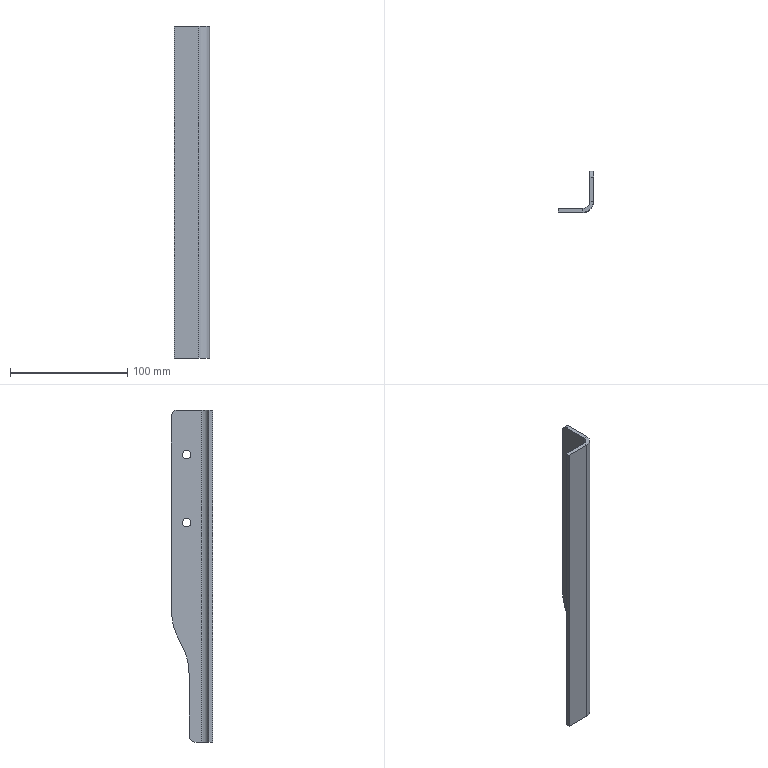Part | SolidWorks | features Fillet 2, FlatPattern 1, ICE 1, SMBaseFlange 1, SheetMetal 1 | 1 solid | 24 faces | box 30 x 35 x 283 mm | volume 48637 mm3 | plane 14 | cylinder 10 | commonest cylinder face diameters 7.2 x4 10 x2 100 x2 12 x1 18.4 x1
STEP:
#1=CARTESIAN_POINT('',(0.,22.,41.8));
#2=VERTEX_POINT('',#1);
#3=CARTESIAN_POINT('',(0.,22.,49.));
#4=VERTEX_POINT('',#3);
#5=CARTESIAN_POINT('',(0.,22.,45.4));
#6=DIRECTION('',(-1.,0.,0.));
#7=DIRECTION('',(0.,0.,1.));
#8=AXIS2_PLACEMENT_3D('',#5,#6,#7);
#9=CIRCLE('',#8,3.6);
#10=EDGE_CURVE('',#2,#4,#9,.T.);
#11=ORIENTED_EDGE('',*,*,#10,.F.);
#12=CARTESIAN_POINT('',(-3.2,22.,41.8));
#13=VERTEX_POINT('',#12);
#14=CARTESIAN_POINT('',(-3.2,22.,41.8));
#15=DIRECTION('',(-1.,0.,0.));
#16=VECTOR('',#15,1000.);
#17=LINE('',#14,#16);
#18=EDGE_CURVE('',#2,#13,#17,.T.);
#19=ORIENTED_EDGE('',*,*,#18,.T.);
#20=CARTESIAN_POINT('',(-3.2,22.,49.));
#21=VERTEX_POINT('',#20);
#22=CARTESIAN_POINT('',(-3.2,22.,45.4));
#23=DIRECTION('',(-1.,0.,0.));
#24=DIRECTION('',(0.,0.,1.));
#25=AXIS2_PLACEMENT_3D('',#22,#23,#24);
#26=CIRCLE('',#25,3.6);
#27=EDGE_CURVE('',#13,#21,#26,.T.);
#28=ORIENTED_EDGE('',*,*,#27,.T.);
#29=CARTESIAN_POINT('',(-3.2,22.,49.));
#30=DIRECTION('',(-1.,0.,0.));
#31=VECTOR('',#30,1000.);
#32=LINE('',#29,#31);
#33=EDGE_CURVE('',#4,#21,#32,.T.);
#34=ORIENTED_EDGE('',*,*,#33,.F.);
#35=EDGE_LOOP('',(#11,#19,#28,#34));
#36=FACE_OUTER_BOUND('',#35,.T.);
#37=CARTESIAN_POINT('',(-3.2,22.,45.4));
#38=DIRECTION('',(-1.,0.,0.));
#39=DIRECTION('',(0.,0.,1.));
#40=AXIS2_PLACEMENT_3D('',#37,#38,#39);
#41=CYLINDRICAL_SURFACE('',#40,3.6);
#42=ADVANCED_FACE('',(#36),#41,.F.);
#43=CARTESIAN_POINT('',(0.,22.,99.8));
#44=VERTEX_POINT('',#43);
#45=CARTESIAN_POINT('',(0.,22.,107.));
#46=VERTEX_POINT('',#45);
#47=CARTESIAN_POINT('',(0.,22.,103.4));
#48=DIRECTION('',(-1.,0.,0.));
#49=DIRECTION('',(0.,0.,1.));
#50=AXIS2_PLACEMENT_3D('',#47,#48,#49);
#51=CIRCLE('',#50,3.6);
#52=EDGE_CURVE('',#44,#46,#51,.T.);
#53=ORIENTED_EDGE('',*,*,#52,.F.);
#54=CARTESIAN_POINT('',(-3.2,22.,99.8));
#55=VERTEX_POINT('',#54);
#56=CARTESIAN_POINT('',(-3.2,22.,99.8));
#57=DIRECTION('',(-1.,0.,0.));
#58=VECTOR('',#57,1000.);
#59=LINE('',#56,#58);
#60=EDGE_CURVE('',#44,#55,#59,.T.);
#61=ORIENTED_EDGE('',*,*,#60,.T.);
#62=CARTESIAN_POINT('',(-3.2,22.,107.));
#63=VERTEX_POINT('',#62);
#64=CARTESIAN_POINT('',(-3.2,22.,103.4));
#65=DIRECTION('',(-1.,0.,0.));
#66=DIRECTION('',(0.,0.,1.));
#67=AXIS2_PLACEMENT_3D('',#64,#65,#66);
#68=CIRCLE('',#67,3.6);
#69=EDGE_CURVE('',#55,#63,#68,.T.);
#70=ORIENTED_EDGE('',*,*,#69,.T.);
#71=CARTESIAN_POINT('',(-3.2,22.,107.));
#72=DIRECTION('',(-1.,0.,0.));
#73=VECTOR('',#72,1000.);
#74=LINE('',#71,#73);
#75=EDGE_CURVE('',#46,#63,#74,.T.);
#76=ORIENTED_EDGE('',*,*,#75,.F.);
#77=EDGE_LOOP('',(#53,#61,#70,#76));
#78=FACE_OUTER_BOUND('',#77,.T.);
#79=CARTESIAN_POINT('',(-3.2,22.,103.4));
#80=DIRECTION('',(-1.,0.,0.));
#81=DIRECTION('',(0.,0.,1.));
#82=AXIS2_PLACEMENT_3D('',#79,#80,#81);
#83=CYLINDRICAL_SURFACE('',#82,3.6);
#84=ADVANCED_FACE('',(#78),#83,.F.);
#85=CARTESIAN_POINT('',(-3.2,9.2,-141.5));
#86=VERTEX_POINT('',#85);
#87=CARTESIAN_POINT('',(-3.2,15.,-141.5));
#88=VERTEX_POINT('',#87);
#89=CARTESIAN_POINT('',(-3.2,0.,-141.5));
#90=DIRECTION('',(0.,1.,0.));
#91=VECTOR('',#90,1000.);
#92=LINE('',#89,#91);
#93=EDGE_CURVE('',#86,#88,#92,.T.);
#94=ORIENTED_EDGE('',*,*,#93,.T.);
#95=CARTESIAN_POINT('',(0.,15.,-141.5));
#96=VERTEX_POINT('',#95);
#97=CARTESIAN_POINT('',(-9.2,15.,-141.5));
#98=DIRECTION('',(1.,0.,0.));
#99=VECTOR('',#98,1000.);
#100=LINE('',#97,#99);
#101=EDGE_CURVE('',#88,#96,#100,.T.);
#102=ORIENTED_EDGE('',*,*,#101,.T.);
#103=CARTESIAN_POINT('',(0.,9.2,-141.5));
#104=VERTEX_POINT('',#103);
#105=CARTESIAN_POINT('',(0.,0.,-141.5));
#106=DIRECTION('',(0.,1.,0.));
#107=VECTOR('',#106,1000.);
#108=LINE('',#105,#107);
#109=EDGE_CURVE('',#104,#96,#108,.T.);
#110=ORIENTED_EDGE('',*,*,#109,.F.);
#111=CARTESIAN_POINT('',(0.,9.2,-141.5));
#112=DIRECTION('',(-1.,0.,0.));
#113=VECTOR('',#112,1000.);
#114=LINE('',#111,#113);
#115=EDGE_CURVE('',#104,#86,#114,.T.);
#116=ORIENTED_EDGE('',*,*,#115,.T.);
#117=EDGE_LOOP('',(#94,#102,#110,#116));
#118=FACE_OUTER_BOUND('',#117,.T.);
#119=CARTESIAN_POINT('',(-9.2,3.2,-141.5));
#120=DIRECTION('',(0.,0.,-1.));
#121=DIRECTION('',(-1.,0.,0.));
#122=AXIS2_PLACEMENT_3D('',#119,#120,#121);
#123=PLANE('',#122);
#124=ADVANCED_FACE('',(#118),#123,.T.);
#125=CARTESIAN_POINT('',(-3.2,35.,136.5));
#126=VERTEX_POINT('',#125);
#127=CARTESIAN_POINT('',(-3.2,35.,-29.697));
#128=VERTEX_POINT('',#127);
#129=CARTESIAN_POINT('',(-3.2,35.,141.5));
#130=DIRECTION('',(0.,0.,-1.));
#131=VECTOR('',#130,1000.);
#132=LINE('',#129,#131);
#133=EDGE_CURVE('',#126,#128,#132,.T.);
#134=ORIENTED_EDGE('',*,*,#133,.F.);
#135=CARTESIAN_POINT('',(0.,35.,136.5));
#136=VERTEX_POINT('',#135);
#137=CARTESIAN_POINT('',(-3.2,35.,136.5));
#138=DIRECTION('',(1.,0.,0.));
#139=VECTOR('',#138,1000.);
#140=LINE('',#137,#139);
#141=EDGE_CURVE('',#126,#136,#140,.T.);
#142=ORIENTED_EDGE('',*,*,#141,.T.);
#143=CARTESIAN_POINT('',(0.,35.,-29.697));
#144=VERTEX_POINT('',#143);
#145=CARTESIAN_POINT('',(0.,35.,141.5));
#146=DIRECTION('',(0.,0.,-1.));
#147=VECTOR('',#146,1000.);
#148=LINE('',#145,#147);
#149=EDGE_CURVE('',#136,#144,#148,.T.);
#150=ORIENTED_EDGE('',*,*,#149,.T.);
#151=CARTESIAN_POINT('',(-3.2,35.,-29.697));
#152=DIRECTION('',(-1.,0.,0.));
#153=VECTOR('',#152,1000.);
#154=LINE('',#151,#153);
#155=EDGE_CURVE('',#144,#128,#154,.T.);
#156=ORIENTED_EDGE('',*,*,#155,.T.);
#157=EDGE_LOOP('',(#134,#142,#150,#156));
#158=FACE_OUTER_BOUND('',#157,.T.);
#159=CARTESIAN_POINT('',(-3.2,35.,141.5));
#160=DIRECTION('',(0.,1.,0.));
#161=DIRECTION('',(0.,0.,1.));
#162=AXIS2_PLACEMENT_3D('',#159,#160,#161);
#163=PLANE('',#162);
#164=ADVANCED_FACE('',(#158),#163,.T.);
#165=CARTESIAN_POINT('',(-9.2,0.,141.5));
#166=VERTEX_POINT('',#165);
#167=CARTESIAN_POINT('',(-9.2,3.2,141.5));
#168=VERTEX_POINT('',#167);
#169=CARTESIAN_POINT('',(-9.2,0.,141.5));
#170=DIRECTION('',(0.,1.,0.));
#171=VECTOR('',#170,1000.);
#172=LINE('',#169,#171);
#173=EDGE_CURVE('',#166,#168,#172,.T.);
#174=ORIENTED_EDGE('',*,*,#173,.F.);
#175=CARTESIAN_POINT('',(0.,9.2,141.5));
#176=VERTEX_POINT('',#175);
#177=CARTESIAN_POINT('',(-9.2,9.2,141.5));
#178=DIRECTION('',(0.,0.,1.));
#179=DIRECTION('',(-1.,0.,0.));
#180=AXIS2_PLACEMENT_3D('',#177,#178,#179);
#181=CIRCLE('',#180,9.2);
#182=EDGE_CURVE('',#166,#176,#181,.T.);
#183=ORIENTED_EDGE('',*,*,#182,.T.);
#184=CARTESIAN_POINT('',(-3.2,9.2,141.5));
#185=VERTEX_POINT('',#184);
#186=CARTESIAN_POINT('',(-3.2,9.2,141.5));
#187=DIRECTION('',(1.,0.,0.));
#188=VECTOR('',#187,1000.);
#189=LINE('',#186,#188);
#190=EDGE_CURVE('',#185,#176,#189,.T.);
#191=ORIENTED_EDGE('',*,*,#190,.F.);
#192=CARTESIAN_POINT('',(-9.2,9.2,141.5));
#193=DIRECTION('',(0.,0.,1.));
#194=DIRECTION('',(1.,0.,0.));
#195=AXIS2_PLACEMENT_3D('',#192,#193,#194);
#196=CIRCLE('',#195,6.);
#197=EDGE_CURVE('',#168,#185,#196,.T.);
#198=ORIENTED_EDGE('',*,*,#197,.F.);
#199=EDGE_LOOP('',(#174,#183,#191,#198));
#200=FACE_OUTER_BOUND('',#199,.T.);
#201=CARTESIAN_POINT('',(-9.2,0.,141.5));
#202=DIRECTION('',(0.,0.,1.));
#203=DIRECTION('',(1.,0.,0.));
#204=AXIS2_PLACEMENT_3D('',#201,#202,#203);
#205=PLANE('',#204);
#206=ADVANCED_FACE('',(#200),#205,.T.);
#207=CARTESIAN_POINT('',(-30.,0.,141.5));
#208=VERTEX_POINT('',#207);
#209=CARTESIAN_POINT('',(0.,0.,141.5));
#210=DIRECTION('',(1.,0.,0.));
#211=VECTOR('',#210,1000.);
#212=LINE('',#209,#211);
#213=EDGE_CURVE('',#208,#166,#212,.T.);
#214=ORIENTED_EDGE('',*,*,#213,.T.);
#215=ORIENTED_EDGE('',*,*,#173,.T.);
#216=CARTESIAN_POINT('',(-30.,3.2,141.5));
#217=VERTEX_POINT('',#216);
#218=CARTESIAN_POINT('',(0.,3.2,141.5));
#219=DIRECTION('',(1.,0.,0.));
#220=VECTOR('',#219,1000.);
#221=LINE('',#218,#220);
#222=EDGE_CURVE('',#217,#168,#221,.T.);
#223=ORIENTED_EDGE('',*,*,#222,.F.);
#224=CARTESIAN_POINT('',(-30.,0.,141.5));
#225=DIRECTION('',(0.,1.,0.));
#226=VECTOR('',#225,1000.);
#227=LINE('',#224,#226);
#228=EDGE_CURVE('',#208,#217,#227,.T.);
#229=ORIENTED_EDGE('',*,*,#228,.F.);
#230=EDGE_LOOP('',(#214,#215,#223,#229));
#231=FACE_OUTER_BOUND('',#230,.T.);
#232=CARTESIAN_POINT('',(-3.2,9.2,141.5));
#233=DIRECTION('',(0.,0.,1.));
#234=DIRECTION('',(1.,0.,0.));
#235=AXIS2_PLACEMENT_3D('',#232,#233,#234);
#236=PLANE('',#235);
#237=ADVANCED_FACE('',(#231),#236,.T.);
#238=ORIENTED_EDGE('',*,*,#115,.F.);
#239=CARTESIAN_POINT('',(-9.2,0.,-141.5));
#240=VERTEX_POINT('',#239);
#241=CARTESIAN_POINT('',(-9.2,9.2,-141.5));
#242=DIRECTION('',(0.,0.,1.));
#243=DIRECTION('',(-1.,0.,0.));
#244=AXIS2_PLACEMENT_3D('',#241,#242,#243);
#245=CIRCLE('',#244,9.2);
#246=EDGE_CURVE('',#240,#104,#245,.T.);
#247=ORIENTED_EDGE('',*,*,#246,.F.);
#248=CARTESIAN_POINT('',(-9.2,3.2,-141.5));
#249=VERTEX_POINT('',#248);
#250=CARTESIAN_POINT('',(-9.2,3.2,-141.5));
#251=DIRECTION('',(0.,-1.,0.));
#252=VECTOR('',#251,1000.);
#253=LINE('',#250,#252);
#254=EDGE_CURVE('',#249,#240,#253,.T.);
#255=ORIENTED_EDGE('',*,*,#254,.F.);
#256=CARTESIAN_POINT('',(-9.2,9.2,-141.5));
#257=DIRECTION('',(0.,0.,1.));
#258=DIRECTION('',(1.,0.,0.));
#259=AXIS2_PLACEMENT_3D('',#256,#257,#258);
#260=CIRCLE('',#259,6.);
#261=EDGE_CURVE('',#249,#86,#260,.T.);
#262=ORIENTED_EDGE('',*,*,#261,.T.);
#263=EDGE_LOOP('',(#238,#247,#255,#262));
#264=FACE_OUTER_BOUND('',#263,.T.);
#265=CARTESIAN_POINT('',(0.,9.2,-141.5));
#266=DIRECTION('',(0.,0.,-1.));
#267=DIRECTION('',(-1.,0.,0.));
#268=AXIS2_PLACEMENT_3D('',#265,#266,#267);
#269=PLANE('',#268);
#270=ADVANCED_FACE('',(#264),#269,.T.);
#271=ORIENTED_EDGE('',*,*,#109,.T.);
#272=CARTESIAN_POINT('',(0.,20.,-136.5));
#273=VERTEX_POINT('',#272);
#274=CARTESIAN_POINT('',(0.,15.,-136.5));
#275=DIRECTION('',(1.,0.,0.));
#276=DIRECTION('',(0.,0.,1.));
#277=AXIS2_PLACEMENT_3D('',#274,#275,#276);
#278=CIRCLE('',#277,5.);
#279=EDGE_CURVE('',#96,#273,#278,.T.);
#280=ORIENTED_EDGE('',*,*,#279,.T.);
#281=CARTESIAN_POINT('',(0.,20.,-83.303));
#282=VERTEX_POINT('',#281);
#283=CARTESIAN_POINT('',(0.,20.,141.5));
#284=DIRECTION('',(0.,0.,1.));
#285=VECTOR('',#284,1000.);
#286=LINE('',#283,#285);
#287=EDGE_CURVE('',#273,#282,#286,.T.);
#288=ORIENTED_EDGE('',*,*,#287,.T.);
#289=CARTESIAN_POINT('',(0.,25.279,-60.943));
#290=VERTEX_POINT('',#289);
#291=CARTESIAN_POINT('',(0.,70.,-83.303));
#292=DIRECTION('',(-1.,0.,0.));
#293=DIRECTION('',(0.,0.,1.));
#294=AXIS2_PLACEMENT_3D('',#291,#292,#293);
#295=CIRCLE('',#294,50.);
#296=EDGE_CURVE('',#282,#290,#295,.T.);
#297=ORIENTED_EDGE('',*,*,#296,.T.);
#298=CARTESIAN_POINT('',(0.,29.721,-52.057));
#299=VERTEX_POINT('',#298);
#300=CARTESIAN_POINT('',(0.,101.2,90.9));
#301=DIRECTION('',(0.,0.4472,0.8944));
#302=VECTOR('',#301,1000.);
#303=LINE('',#300,#302);
#304=EDGE_CURVE('',#290,#299,#303,.T.);
#305=ORIENTED_EDGE('',*,*,#304,.T.);
#306=CARTESIAN_POINT('',(0.,-15.,-29.697));
#307=DIRECTION('',(1.,0.,0.));
#308=DIRECTION('',(0.,0.,1.));
#309=AXIS2_PLACEMENT_3D('',#306,#307,#308);
#310=CIRCLE('',#309,50.);
#311=EDGE_CURVE('',#299,#144,#310,.T.);
#312=ORIENTED_EDGE('',*,*,#311,.T.);
#313=ORIENTED_EDGE('',*,*,#149,.F.);
#314=CARTESIAN_POINT('',(0.,30.,141.5));
#315=VERTEX_POINT('',#314);
#316=CARTESIAN_POINT('',(0.,30.,136.5));
#317=DIRECTION('',(1.,0.,0.));
#318=DIRECTION('',(0.,0.,1.));
#319=AXIS2_PLACEMENT_3D('',#316,#317,#318);
#320=CIRCLE('',#319,5.);
#321=EDGE_CURVE('',#136,#315,#320,.T.);
#322=ORIENTED_EDGE('',*,*,#321,.T.);
#323=CARTESIAN_POINT('',(0.,0.,141.5));
#324=DIRECTION('',(0.,1.,0.));
#325=VECTOR('',#324,1000.);
#326=LINE('',#323,#325);
#327=EDGE_CURVE('',#176,#315,#326,.T.);
#328=ORIENTED_EDGE('',*,*,#327,.F.);
#329=CARTESIAN_POINT('',(0.,9.2,141.5));
#330=DIRECTION('',(0.,0.,-1.));
#331=VECTOR('',#330,1000.);
#332=LINE('',#329,#331);
#333=EDGE_CURVE('',#176,#104,#332,.T.);
#334=ORIENTED_EDGE('',*,*,#333,.T.);
#335=EDGE_LOOP('',(#271,#280,#288,#297,#305,#312,#313,#322,#328,#334));
#336=FACE_OUTER_BOUND('',#335,.T.);
#337=CARTESIAN_POINT('',(0.,22.,45.4));
#338=DIRECTION('',(-1.,0.,0.));
#339=DIRECTION('',(0.,0.,1.));
#340=AXIS2_PLACEMENT_3D('',#337,#338,#339);
#341=CIRCLE('',#340,3.6);
#342=EDGE_CURVE('',#4,#2,#341,.T.);
#343=ORIENTED_EDGE('',*,*,#342,.T.);
#344=ORIENTED_EDGE('',*,*,#10,.T.);
#345=EDGE_LOOP('',(#343,#344));
#346=FACE_BOUND('',#345,.T.);
#347=CARTESIAN_POINT('',(0.,22.,103.4));
#348=DIRECTION('',(-1.,0.,0.));
#349=DIRECTION('',(0.,0.,1.));
#350=AXIS2_PLACEMENT_3D('',#347,#348,#349);
#351=CIRCLE('',#350,3.6);
#352=EDGE_CURVE('',#46,#44,#351,.T.);
#353=ORIENTED_EDGE('',*,*,#352,.T.);
#354=ORIENTED_EDGE('',*,*,#52,.T.);
#355=EDGE_LOOP('',(#353,#354));
#356=FACE_BOUND('',#355,.T.);
#357=CARTESIAN_POINT('',(0.,0.,141.5));
#358=DIRECTION('',(-1.,0.,0.));
#359=DIRECTION('',(0.,0.,1.));
#360=AXIS2_PLACEMENT_3D('',#357,#358,#359);
#361=PLANE('',#360);
#362=ADVANCED_FACE('',(#336,#346,#356),#361,.F.);
#363=CARTESIAN_POINT('',(-3.2,22.,45.4));
#364=DIRECTION('',(-1.,0.,0.));
#365=DIRECTION('',(0.,0.,1.));
#366=AXIS2_PLACEMENT_3D('',#363,#364,#365);
#367=CIRCLE('',#366,3.6);
#368=EDGE_CURVE('',#21,#13,#367,.T.);
#369=ORIENTED_EDGE('',*,*,#368,.F.);
#370=ORIENTED_EDGE('',*,*,#27,.F.);
#371=EDGE_LOOP('',(#369,#370));
#372=FACE_BOUND('',#371,.T.);
#373=CARTESIAN_POINT('',(-3.2,22.,103.4));
#374=DIRECTION('',(-1.,0.,0.));
#375=DIRECTION('',(0.,0.,1.));
#376=AXIS2_PLACEMENT_3D('',#373,#374,#375);
#377=CIRCLE('',#376,3.6);
#378=EDGE_CURVE('',#63,#55,#377,.T.);
#379=ORIENTED_EDGE('',*,*,#378,.F.);
#380=ORIENTED_EDGE('',*,*,#69,.F.);
#381=EDGE_LOOP('',(#379,#380));
#382=FACE_BOUND('',#381,.T.);
#383=CARTESIAN_POINT('',(-3.2,20.,-136.5));
#384=VERTEX_POINT('',#383);
#385=CARTESIAN_POINT('',(-3.2,20.,-83.303));
#386=VERTEX_POINT('',#385);
#387=CARTESIAN_POINT('',(-3.2,20.,141.5));
#388=DIRECTION('',(0.,0.,1.));
#389=VECTOR('',#388,1000.);
#390=LINE('',#387,#389);
#391=EDGE_CURVE('',#384,#386,#390,.T.);
#392=ORIENTED_EDGE('',*,*,#391,.F.);
#393=CARTESIAN_POINT('',(-3.2,15.,-136.5));
#394=DIRECTION('',(-1.,0.,0.));
#395=DIRECTION('',(0.,0.,1.));
#396=AXIS2_PLACEMENT_3D('',#393,#394,#395);
#397=CIRCLE('',#396,5.);
#398=EDGE_CURVE('',#384,#88,#397,.T.);
#399=ORIENTED_EDGE('',*,*,#398,.T.);
#400=ORIENTED_EDGE('',*,*,#93,.F.);
#401=CARTESIAN_POINT('',(-3.2,9.2,141.5));
#402=DIRECTION('',(0.,0.,-1.));
#403=VECTOR('',#402,1000.);
#404=LINE('',#401,#403);
#405=EDGE_CURVE('',#185,#86,#404,.T.);
#406=ORIENTED_EDGE('',*,*,#405,.F.);
#407=CARTESIAN_POINT('',(-3.2,30.,141.5));
#408=VERTEX_POINT('',#407);
#409=CARTESIAN_POINT('',(-3.2,0.,141.5));
#410=DIRECTION('',(0.,1.,0.));
#411=VECTOR('',#410,1000.);
#412=LINE('',#409,#411);
#413=EDGE_CURVE('',#185,#408,#412,.T.);
#414=ORIENTED_EDGE('',*,*,#413,.T.);
#415=CARTESIAN_POINT('',(-3.2,30.,136.5));
#416=DIRECTION('',(-1.,0.,0.));
#417=DIRECTION('',(0.,0.,1.));
#418=AXIS2_PLACEMENT_3D('',#415,#416,#417);
#419=CIRCLE('',#418,5.);
#420=EDGE_CURVE('',#408,#126,#419,.T.);
#421=ORIENTED_EDGE('',*,*,#420,.T.);
#422=ORIENTED_EDGE('',*,*,#133,.T.);
#423=CARTESIAN_POINT('',(-3.2,29.721,-52.057));
#424=VERTEX_POINT('',#423);
#425=CARTESIAN_POINT('',(-3.2,-15.,-29.697));
#426=DIRECTION('',(-1.,0.,0.));
#427=DIRECTION('',(0.,0.,1.));
#428=AXIS2_PLACEMENT_3D('',#425,#426,#427);
#429=CIRCLE('',#428,50.);
#430=EDGE_CURVE('',#128,#424,#429,.T.);
#431=ORIENTED_EDGE('',*,*,#430,.T.);
#432=CARTESIAN_POINT('',(-3.2,25.279,-60.943));
#433=VERTEX_POINT('',#432);
#434=CARTESIAN_POINT('',(-3.2,101.2,90.9));
#435=DIRECTION('',(0.,0.4472,0.8944));
#436=VECTOR('',#435,1000.);
#437=LINE('',#434,#436);
#438=EDGE_CURVE('',#433,#424,#437,.T.);
#439=ORIENTED_EDGE('',*,*,#438,.F.);
#440=CARTESIAN_POINT('',(-3.2,70.,-83.303));
#441=DIRECTION('',(1.,0.,0.));
#442=DIRECTION('',(0.,0.,1.));
#443=AXIS2_PLACEMENT_3D('',#440,#441,#442);
#444=CIRCLE('',#443,50.);
#445=EDGE_CURVE('',#433,#386,#444,.T.);
#446=ORIENTED_EDGE('',*,*,#445,.T.);
#447=EDGE_LOOP('',(#392,#399,#400,#406,#414,#421,#422,#431,#439,#446));
#448=FACE_OUTER_BOUND('',#447,.T.);
#449=CARTESIAN_POINT('',(-3.2,0.,141.5));
#450=DIRECTION('',(-1.,0.,0.));
#451=DIRECTION('',(0.,0.,1.));
#452=AXIS2_PLACEMENT_3D('',#449,#450,#451);
#453=PLANE('',#452);
#454=ADVANCED_FACE('',(#372,#382,#448),#453,.T.);
#455=ORIENTED_EDGE('',*,*,#261,.F.);
#456=CARTESIAN_POINT('',(-9.2,3.2,141.5));
#457=DIRECTION('',(0.,0.,-1.));
#458=VECTOR('',#457,1000.);
#459=LINE('',#456,#458);
#460=EDGE_CURVE('',#168,#249,#459,.T.);
#461=ORIENTED_EDGE('',*,*,#460,.F.);
#462=ORIENTED_EDGE('',*,*,#197,.T.);
#463=ORIENTED_EDGE('',*,*,#405,.T.);
#464=EDGE_LOOP('',(#455,#461,#462,#463));
#465=FACE_OUTER_BOUND('',#464,.T.);
#466=CARTESIAN_POINT('',(-9.2,9.2,141.5));
#467=DIRECTION('',(0.,0.,-1.));
#468=DIRECTION('',(-1.,0.,0.));
#469=AXIS2_PLACEMENT_3D('',#466,#467,#468);
#470=CYLINDRICAL_SURFACE('',#469,6.);
#471=ADVANCED_FACE('',(#465),#470,.F.);
#472=CARTESIAN_POINT('',(-30.,3.2,-141.5));
#473=VERTEX_POINT('',#472);
#474=CARTESIAN_POINT('',(0.,3.2,-141.5));
#475=DIRECTION('',(1.,0.,0.));
#476=VECTOR('',#475,1000.);
#477=LINE('',#474,#476);
#478=EDGE_CURVE('',#473,#249,#477,.T.);
#479=ORIENTED_EDGE('',*,*,#478,.F.);
#480=CARTESIAN_POINT('',(-30.,3.2,141.5));
#481=DIRECTION('',(0.,0.,-1.));
#482=VECTOR('',#481,1000.);
#483=LINE('',#480,#482);
#484=EDGE_CURVE('',#217,#473,#483,.T.);
#485=ORIENTED_EDGE('',*,*,#484,.F.);
#486=ORIENTED_EDGE('',*,*,#222,.T.);
#487=ORIENTED_EDGE('',*,*,#460,.T.);
#488=EDGE_LOOP('',(#479,#485,#486,#487));
#489=FACE_OUTER_BOUND('',#488,.T.);
#490=CARTESIAN_POINT('',(0.,3.2,141.5));
#491=DIRECTION('',(0.,1.,0.));
#492=DIRECTION('',(0.,0.,1.));
#493=AXIS2_PLACEMENT_3D('',#490,#491,#492);
#494=PLANE('',#493);
#495=ADVANCED_FACE('',(#489),#494,.T.);
#496=CARTESIAN_POINT('',(-30.,0.,-141.5));
#497=VERTEX_POINT('',#496);
#498=CARTESIAN_POINT('',(-30.,0.,-141.5));
#499=DIRECTION('',(0.,1.,0.));
#500=VECTOR('',#499,1000.);
#501=LINE('',#498,#500);
#502=EDGE_CURVE('',#497,#473,#501,.T.);
#503=ORIENTED_EDGE('',*,*,#502,.F.);
#504=CARTESIAN_POINT('',(-30.,0.,141.5));
#505=DIRECTION('',(0.,0.,-1.));
#506=VECTOR('',#505,1000.);
#507=LINE('',#504,#506);
#508=EDGE_CURVE('',#208,#497,#507,.T.);
#509=ORIENTED_EDGE('',*,*,#508,.F.);
#510=ORIENTED_EDGE('',*,*,#228,.T.);
#511=ORIENTED_EDGE('',*,*,#484,.T.);
#512=EDGE_LOOP('',(#503,#509,#510,#511));
#513=FACE_OUTER_BOUND('',#512,.T.);
#514=CARTESIAN_POINT('',(-30.,0.,141.5));
#515=DIRECTION('',(-1.,0.,0.));
#516=DIRECTION('',(0.,0.,1.));
#517=AXIS2_PLACEMENT_3D('',#514,#515,#516);
#518=PLANE('',#517);
#519=ADVANCED_FACE('',(#513),#518,.T.);
#520=CARTESIAN_POINT('',(0.,0.,-141.5));
#521=DIRECTION('',(1.,0.,0.));
#522=VECTOR('',#521,1000.);
#523=LINE('',#520,#522);
#524=EDGE_CURVE('',#497,#240,#523,.T.);
#525=ORIENTED_EDGE('',*,*,#524,.T.);
#526=CARTESIAN_POINT('',(-9.2,0.,141.5));
#527=DIRECTION('',(0.,0.,-1.));
#528=VECTOR('',#527,1000.);
#529=LINE('',#526,#528);
#530=EDGE_CURVE('',#166,#240,#529,.T.);
#531=ORIENTED_EDGE('',*,*,#530,.F.);
#532=ORIENTED_EDGE('',*,*,#213,.F.);
#533=ORIENTED_EDGE('',*,*,#508,.T.);
#534=EDGE_LOOP('',(#525,#531,#532,#533));
#535=FACE_OUTER_BOUND('',#534,.T.);
#536=CARTESIAN_POINT('',(0.,0.,141.5));
#537=DIRECTION('',(0.,1.,0.));
#538=DIRECTION('',(0.,0.,1.));
#539=AXIS2_PLACEMENT_3D('',#536,#537,#538);
#540=PLANE('',#539);
#541=ADVANCED_FACE('',(#535),#540,.F.);
#542=ORIENTED_EDGE('',*,*,#246,.T.);
#543=ORIENTED_EDGE('',*,*,#333,.F.);
#544=ORIENTED_EDGE('',*,*,#182,.F.);
#545=ORIENTED_EDGE('',*,*,#530,.T.);
#546=EDGE_LOOP('',(#542,#543,#544,#545));
#547=FACE_OUTER_BOUND('',#546,.T.);
#548=CARTESIAN_POINT('',(-9.2,9.2,141.5));
#549=DIRECTION('',(0.,0.,-1.));
#550=DIRECTION('',(-1.,0.,0.));
#551=AXIS2_PLACEMENT_3D('',#548,#549,#550);
#552=CYLINDRICAL_SURFACE('',#551,9.2);
#553=ADVANCED_FACE('',(#547),#552,.T.);
#554=ORIENTED_EDGE('',*,*,#327,.T.);
#555=CARTESIAN_POINT('',(-9.2,30.,141.5));
#556=DIRECTION('',(-1.,0.,0.));
#557=VECTOR('',#556,1000.);
#558=LINE('',#555,#557);
#559=EDGE_CURVE('',#315,#408,#558,.T.);
#560=ORIENTED_EDGE('',*,*,#559,.T.);
#561=ORIENTED_EDGE('',*,*,#413,.F.);
#562=ORIENTED_EDGE('',*,*,#190,.T.);
#563=EDGE_LOOP('',(#554,#560,#561,#562));
#564=FACE_OUTER_BOUND('',#563,.T.);
#565=CARTESIAN_POINT('',(-9.2,9.2,141.5));
#566=DIRECTION('',(0.,0.,1.));
#567=DIRECTION('',(1.,0.,0.));
#568=AXIS2_PLACEMENT_3D('',#565,#566,#567);
#569=PLANE('',#568);
#570=ADVANCED_FACE('',(#564),#569,.T.);
#571=ORIENTED_EDGE('',*,*,#478,.T.);
#572=ORIENTED_EDGE('',*,*,#254,.T.);
#573=ORIENTED_EDGE('',*,*,#524,.F.);
#574=ORIENTED_EDGE('',*,*,#502,.T.);
#575=EDGE_LOOP('',(#571,#572,#573,#574));
#576=FACE_OUTER_BOUND('',#575,.T.);
#577=CARTESIAN_POINT('',(-9.2,9.2,-141.5));
#578=DIRECTION('',(0.,0.,1.));
#579=DIRECTION('',(1.,0.,0.));
#580=AXIS2_PLACEMENT_3D('',#577,#578,#579);
#581=PLANE('',#580);
#582=ADVANCED_FACE('',(#576),#581,.F.);
#583=ORIENTED_EDGE('',*,*,#60,.F.);
#584=ORIENTED_EDGE('',*,*,#352,.F.);
#585=ORIENTED_EDGE('',*,*,#75,.T.);
#586=ORIENTED_EDGE('',*,*,#378,.T.);
#587=EDGE_LOOP('',(#583,#584,#585,#586));
#588=FACE_OUTER_BOUND('',#587,.T.);
#589=CARTESIAN_POINT('',(-3.2,22.,103.4));
#590=DIRECTION('',(-1.,0.,0.));
#591=DIRECTION('',(0.,0.,1.));
#592=AXIS2_PLACEMENT_3D('',#589,#590,#591);
#593=CYLINDRICAL_SURFACE('',#592,3.6);
#594=ADVANCED_FACE('',(#588),#593,.F.);
#595=ORIENTED_EDGE('',*,*,#18,.F.);
#596=ORIENTED_EDGE('',*,*,#342,.F.);
#597=ORIENTED_EDGE('',*,*,#33,.T.);
#598=ORIENTED_EDGE('',*,*,#368,.T.);
#599=EDGE_LOOP('',(#595,#596,#597,#598));
#600=FACE_OUTER_BOUND('',#599,.T.);
#601=CARTESIAN_POINT('',(-3.2,22.,45.4));
#602=DIRECTION('',(-1.,0.,0.));
#603=DIRECTION('',(0.,0.,1.));
#604=AXIS2_PLACEMENT_3D('',#601,#602,#603);
#605=CYLINDRICAL_SURFACE('',#604,3.6);
#606=ADVANCED_FACE('',(#600),#605,.F.);
#607=ORIENTED_EDGE('',*,*,#304,.F.);
#608=CARTESIAN_POINT('',(-3.2,25.279,-60.943));
#609=DIRECTION('',(-1.,0.,0.));
#610=VECTOR('',#609,1000.);
#611=LINE('',#608,#610);
#612=EDGE_CURVE('',#290,#433,#611,.T.);
#613=ORIENTED_EDGE('',*,*,#612,.T.);
#614=ORIENTED_EDGE('',*,*,#438,.T.);
#615=CARTESIAN_POINT('',(-3.2,29.721,-52.057));
#616=DIRECTION('',(1.,0.,0.));
#617=VECTOR('',#616,1000.);
#618=LINE('',#615,#617);
#619=EDGE_CURVE('',#424,#299,#618,.T.);
#620=ORIENTED_EDGE('',*,*,#619,.T.);
#621=EDGE_LOOP('',(#607,#613,#614,#620));
#622=FACE_OUTER_BOUND('',#621,.T.);
#623=CARTESIAN_POINT('',(-3.2,101.2,90.9));
#624=DIRECTION('',(0.,-0.8944,0.4472));
#625=DIRECTION('',(0.,0.4472,0.8944));
#626=AXIS2_PLACEMENT_3D('',#623,#624,#625);
#627=PLANE('',#626);
#628=ADVANCED_FACE('',(#622),#627,.F.);
#629=ORIENTED_EDGE('',*,*,#287,.F.);
#630=CARTESIAN_POINT('',(-3.2,20.,-136.5));
#631=DIRECTION('',(-1.,0.,0.));
#632=VECTOR('',#631,1000.);
#633=LINE('',#630,#632);
#634=EDGE_CURVE('',#273,#384,#633,.T.);
#635=ORIENTED_EDGE('',*,*,#634,.T.);
#636=ORIENTED_EDGE('',*,*,#391,.T.);
#637=CARTESIAN_POINT('',(0.,20.,-83.303));
#638=DIRECTION('',(1.,0.,0.));
#639=VECTOR('',#638,1000.);
#640=LINE('',#637,#639);
#641=EDGE_CURVE('',#386,#282,#640,.T.);
#642=ORIENTED_EDGE('',*,*,#641,.T.);
#643=EDGE_LOOP('',(#629,#635,#636,#642));
#644=FACE_OUTER_BOUND('',#643,.T.);
#645=CARTESIAN_POINT('',(-3.2,20.,141.5));
#646=DIRECTION('',(0.,-1.,0.));
#647=DIRECTION('',(0.,0.,1.));
#648=AXIS2_PLACEMENT_3D('',#645,#646,#647);
#649=PLANE('',#648);
#650=ADVANCED_FACE('',(#644),#649,.F.);
#651=ORIENTED_EDGE('',*,*,#445,.F.);
#652=ORIENTED_EDGE('',*,*,#612,.F.);
#653=ORIENTED_EDGE('',*,*,#296,.F.);
#654=ORIENTED_EDGE('',*,*,#641,.F.);
#655=EDGE_LOOP('',(#651,#652,#653,#654));
#656=FACE_OUTER_BOUND('',#655,.T.);
#657=CARTESIAN_POINT('',(-3.2,70.,-83.303));
#658=DIRECTION('',(-1.,0.,0.));
#659=DIRECTION('',(0.,0.,1.));
#660=AXIS2_PLACEMENT_3D('',#657,#658,#659);
#661=CYLINDRICAL_SURFACE('',#660,50.);
#662=ADVANCED_FACE('',(#656),#661,.F.);
#663=ORIENTED_EDGE('',*,*,#430,.F.);
#664=ORIENTED_EDGE('',*,*,#155,.F.);
#665=ORIENTED_EDGE('',*,*,#311,.F.);
#666=ORIENTED_EDGE('',*,*,#619,.F.);
#667=EDGE_LOOP('',(#663,#664,#665,#666));
#668=FACE_OUTER_BOUND('',#667,.T.);
#669=CARTESIAN_POINT('',(-3.2,-15.,-29.697));
#670=DIRECTION('',(-1.,0.,0.));
#671=DIRECTION('',(0.,0.,1.));
#672=AXIS2_PLACEMENT_3D('',#669,#670,#671);
#673=CYLINDRICAL_SURFACE('',#672,50.);
#674=ADVANCED_FACE('',(#668),#673,.T.);
#675=ORIENTED_EDGE('',*,*,#398,.F.);
#676=ORIENTED_EDGE('',*,*,#634,.F.);
#677=ORIENTED_EDGE('',*,*,#279,.F.);
#678=ORIENTED_EDGE('',*,*,#101,.F.);
#679=EDGE_LOOP('',(#675,#676,#677,#678));
#680=FACE_OUTER_BOUND('',#679,.T.);
#681=CARTESIAN_POINT('',(-9.2,15.,-136.5));
#682=DIRECTION('',(-1.,0.,0.));
#683=DIRECTION('',(0.,0.,1.));
#684=AXIS2_PLACEMENT_3D('',#681,#682,#683);
#685=CYLINDRICAL_SURFACE('',#684,5.);
#686=ADVANCED_FACE('',(#680),#685,.T.);
#687=ORIENTED_EDGE('',*,*,#420,.F.);
#688=ORIENTED_EDGE('',*,*,#559,.F.);
#689=ORIENTED_EDGE('',*,*,#321,.F.);
#690=ORIENTED_EDGE('',*,*,#141,.F.);
#691=EDGE_LOOP('',(#687,#688,#689,#690));
#692=FACE_OUTER_BOUND('',#691,.T.);
#693=CARTESIAN_POINT('',(-3.2,30.,136.5));
#694=DIRECTION('',(1.,0.,0.));
#695=DIRECTION('',(0.,0.,-1.));
#696=AXIS2_PLACEMENT_3D('',#693,#694,#695);
#697=CYLINDRICAL_SURFACE('',#696,5.);
#698=ADVANCED_FACE('',(#692),#697,.T.);
#699=CLOSED_SHELL('',(#42,#84,#124,#164,#206,#237,#270,#362,#454,#471,#495,#519,#541,#553,#570,#582,#594,#606,#628,#650,#662,#674,#686,#698));
#700=MANIFOLD_SOLID_BREP('',#699);
#701=CARTESIAN_POINT('',(0.,0.,0.));
#702=DIRECTION('',(0.,0.,1.));
#703=DIRECTION('',(1.,0.,0.));
#704=AXIS2_PLACEMENT_3D('',#701,#702,#703);
#705=(LENGTH_UNIT()NAMED_UNIT(*)SI_UNIT(.MILLI.,.METRE.));
#706=UNCERTAINTY_MEASURE_WITH_UNIT(LENGTH_MEASURE(0.00001),#705,'','');
#707=(NAMED_UNIT(*)PLANE_ANGLE_UNIT()SI_UNIT($,.RADIAN.));
#708=(NAMED_UNIT(*)SI_UNIT($,.STERADIAN.)SOLID_ANGLE_UNIT());
#709=(GEOMETRIC_REPRESENTATION_CONTEXT(3)GLOBAL_UNCERTAINTY_ASSIGNED_CONTEXT((#706))GLOBAL_UNIT_ASSIGNED_CONTEXT((#705,#707,#708))REPRESENTATION_CONTEXT('',''));
#710=ADVANCED_BREP_SHAPE_REPRESENTATION('',(#700,#704),#709);